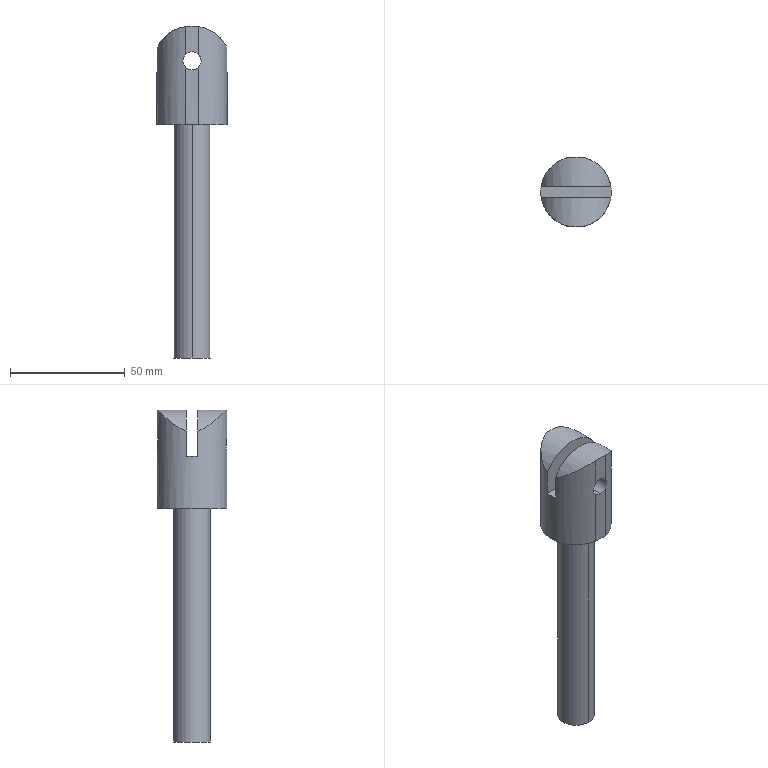Part | NX | features BREP 1 | 1 solid | 20 faces | box 30.734 x 30.163 x 144.78 mm | volume 46621 mm3 | cylinder 11 | plane 9 | commonest cylinder face diameters 7.938 x4 30.734 x3 15.875 x2 34.168 x2
STEP:
#1=CARTESIAN_POINT('',(0.,7.938,-101.6));
#2=VERTEX_POINT('',#1);
#3=CARTESIAN_POINT('',(0.,-7.938,-101.6));
#4=VERTEX_POINT('',#3);
#5=CARTESIAN_POINT('',(0.,0.,-101.6));
#6=DIRECTION('',(0.,0.,-1.));
#7=DIRECTION('',(0.,1.,0.));
#8=AXIS2_PLACEMENT_3D('',#5,#6,#7);
#9=CIRCLE('',#8,7.938);
#10=EDGE_CURVE('',#2,#4,#9,.T.);
#11=ORIENTED_EDGE('',*,*,#10,.T.);
#12=CARTESIAN_POINT('',(0.,0.,-101.6));
#13=DIRECTION('',(0.,0.,-1.));
#14=DIRECTION('',(0.,-1.,0.));
#15=AXIS2_PLACEMENT_3D('',#12,#13,#14);
#16=CIRCLE('',#15,7.938);
#17=EDGE_CURVE('',#4,#2,#16,.T.);
#18=ORIENTED_EDGE('',*,*,#17,.T.);
#19=EDGE_LOOP('',(#11,#18));
#20=FACE_BOUND('',#19,.T.);
#21=CARTESIAN_POINT('',(0.,0.,-101.6));
#22=DIRECTION('',(0.,0.,-1.));
#23=DIRECTION('',(0.,-1.,0.));
#24=AXIS2_PLACEMENT_3D('',#21,#22,#23);
#25=PLANE('',#24);
#26=ADVANCED_FACE('',(#20),#25,.T.);
#27=CARTESIAN_POINT('',(0.,7.938,0.));
#28=VERTEX_POINT('',#27);
#29=CARTESIAN_POINT('',(0.,7.938,0.));
#30=DIRECTION('',(0.,0.,-1.));
#31=VECTOR('',#30,1000.);
#32=LINE('',#29,#31);
#33=EDGE_CURVE('',#2,#28,#32,.F.);
#34=ORIENTED_EDGE('',*,*,#33,.F.);
#35=ORIENTED_EDGE('',*,*,#17,.F.);
#36=CARTESIAN_POINT('',(0.,-7.938,0.));
#37=VERTEX_POINT('',#36);
#38=CARTESIAN_POINT('',(0.,-7.938,0.));
#39=DIRECTION('',(0.,0.,-1.));
#40=VECTOR('',#39,1000.);
#41=LINE('',#38,#40);
#42=EDGE_CURVE('',#4,#37,#41,.F.);
#43=ORIENTED_EDGE('',*,*,#42,.T.);
#44=CARTESIAN_POINT('',(0.,0.,0.));
#45=DIRECTION('',(0.,0.,-1.));
#46=DIRECTION('',(0.,-1.,0.));
#47=AXIS2_PLACEMENT_3D('',#44,#45,#46);
#48=CIRCLE('',#47,7.938);
#49=EDGE_CURVE('',#37,#28,#48,.T.);
#50=ORIENTED_EDGE('',*,*,#49,.T.);
#51=EDGE_LOOP('',(#34,#35,#43,#50));
#52=FACE_BOUND('',#51,.T.);
#53=CARTESIAN_POINT('',(0.,0.,0.));
#54=DIRECTION('',(0.,0.,-1.));
#55=DIRECTION('',(0.,-1.,0.));
#56=AXIS2_PLACEMENT_3D('',#53,#54,#55);
#57=CYLINDRICAL_SURFACE('',#56,7.938);
#58=ADVANCED_FACE('',(#52),#57,.T.);
#59=CARTESIAN_POINT('',(2.95,15.081,0.));
#60=VERTEX_POINT('',#59);
#61=CARTESIAN_POINT('',(-2.95,15.081,0.));
#62=VERTEX_POINT('',#61);
#63=CARTESIAN_POINT('',(2.95,15.081,0.));
#64=DIRECTION('',(-1.,0.,0.));
#65=VECTOR('',#64,1000.);
#66=LINE('',#63,#65);
#67=EDGE_CURVE('',#60,#62,#66,.T.);
#68=ORIENTED_EDGE('',*,*,#67,.F.);
#69=CARTESIAN_POINT('',(15.367,0.,0.));
#70=VERTEX_POINT('',#69);
#71=CARTESIAN_POINT('',(0.,0.,0.));
#72=DIRECTION('',(0.,0.,1.));
#73=DIRECTION('',(0.1919,-0.9814,0.));
#74=AXIS2_PLACEMENT_3D('',#71,#72,#73);
#75=CIRCLE('',#74,15.367);
#76=EDGE_CURVE('',#70,#60,#75,.T.);
#77=ORIENTED_EDGE('',*,*,#76,.F.);
#78=CARTESIAN_POINT('',(2.95,-15.081,0.));
#79=VERTEX_POINT('',#78);
#80=CARTESIAN_POINT('',(0.,0.,0.));
#81=DIRECTION('',(0.,0.,1.));
#82=DIRECTION('',(0.1919,-0.9814,0.));
#83=AXIS2_PLACEMENT_3D('',#80,#81,#82);
#84=CIRCLE('',#83,15.367);
#85=EDGE_CURVE('',#79,#70,#84,.T.);
#86=ORIENTED_EDGE('',*,*,#85,.F.);
#87=CARTESIAN_POINT('',(-2.95,-15.081,0.));
#88=VERTEX_POINT('',#87);
#89=CARTESIAN_POINT('',(-2.95,-15.081,0.));
#90=DIRECTION('',(1.,0.,0.));
#91=VECTOR('',#90,1000.);
#92=LINE('',#89,#91);
#93=EDGE_CURVE('',#88,#79,#92,.T.);
#94=ORIENTED_EDGE('',*,*,#93,.F.);
#95=CARTESIAN_POINT('',(0.,0.,0.));
#96=DIRECTION('',(0.,0.,1.));
#97=DIRECTION('',(-0.1919,0.9814,0.));
#98=AXIS2_PLACEMENT_3D('',#95,#96,#97);
#99=CIRCLE('',#98,15.367);
#100=EDGE_CURVE('',#62,#88,#99,.T.);
#101=ORIENTED_EDGE('',*,*,#100,.F.);
#102=EDGE_LOOP('',(#68,#77,#86,#94,#101));
#103=FACE_BOUND('',#102,.T.);
#104=CARTESIAN_POINT('',(0.,0.,0.));
#105=DIRECTION('',(0.,0.,-1.));
#106=DIRECTION('',(0.,1.,0.));
#107=AXIS2_PLACEMENT_3D('',#104,#105,#106);
#108=CIRCLE('',#107,7.938);
#109=EDGE_CURVE('',#28,#37,#108,.T.);
#110=ORIENTED_EDGE('',*,*,#109,.F.);
#111=ORIENTED_EDGE('',*,*,#49,.F.);
#112=EDGE_LOOP('',(#110,#111));
#113=FACE_BOUND('',#112,.T.);
#114=CARTESIAN_POINT('',(0.,0.,0.));
#115=DIRECTION('',(0.,0.,1.));
#116=DIRECTION('',(1.,0.,0.));
#117=AXIS2_PLACEMENT_3D('',#114,#115,#116);
#118=PLANE('',#117);
#119=ADVANCED_FACE('',(#103,#113),#118,.F.);
#120=CARTESIAN_POINT('',(-2.95,15.081,25.285));
#121=VERTEX_POINT('',#120);
#122=CARTESIAN_POINT('',(-2.95,15.081,0.));
#123=DIRECTION('',(0.,0.,1.));
#124=VECTOR('',#123,1000.);
#125=LINE('',#122,#124);
#126=EDGE_CURVE('',#62,#121,#125,.T.);
#127=ORIENTED_EDGE('',*,*,#126,.F.);
#128=ORIENTED_EDGE('',*,*,#100,.T.);
#129=CARTESIAN_POINT('',(-2.95,-15.081,25.285));
#130=VERTEX_POINT('',#129);
#131=CARTESIAN_POINT('',(-2.95,-15.081,0.));
#132=DIRECTION('',(0.,0.,1.));
#133=VECTOR('',#132,1000.);
#134=LINE('',#131,#133);
#135=EDGE_CURVE('',#88,#130,#134,.T.);
#136=ORIENTED_EDGE('',*,*,#135,.T.);
#137=CARTESIAN_POINT('',(-2.95,-15.081,30.595));
#138=VERTEX_POINT('',#137);
#139=CARTESIAN_POINT('',(-2.95,-15.081,25.285));
#140=CARTESIAN_POINT('',(-3.615,-14.951,26.024));
#141=CARTESIAN_POINT('',(-4.329,-14.739,27.976));
#142=CARTESIAN_POINT('',(-3.601,-14.954,29.872));
#143=CARTESIAN_POINT('',(-2.95,-15.081,30.595));
#144=B_SPLINE_CURVE_WITH_KNOTS('',3,(#139,#140,#141,#142,#143),.UNSPECIFIED.,.F.,.F.,(4,1,4),(0.,0.5,1.),.UNSPECIFIED.);
#145=EDGE_CURVE('',#130,#138,#144,.T.);
#146=ORIENTED_EDGE('',*,*,#145,.T.);
#147=CARTESIAN_POINT('',(-2.95,-15.081,42.923));
#148=VERTEX_POINT('',#147);
#149=CARTESIAN_POINT('',(-2.95,-15.081,30.595));
#150=DIRECTION('',(0.,0.,1.));
#151=VECTOR('',#150,1000.);
#152=LINE('',#149,#151);
#153=EDGE_CURVE('',#138,#148,#152,.T.);
#154=ORIENTED_EDGE('',*,*,#153,.T.);
#155=CARTESIAN_POINT('',(-15.156,-2.54,33.981));
#156=VERTEX_POINT('',#155);
#157=CARTESIAN_POINT('',(-2.95,-15.081,42.923));
#158=CARTESIAN_POINT('',(-3.728,-14.929,42.787));
#159=CARTESIAN_POINT('',(-5.275,-14.509,42.408));
#160=CARTESIAN_POINT('',(-7.248,-13.592,41.602));
#161=CARTESIAN_POINT('',(-8.585,-12.765,40.88));
#162=CARTESIAN_POINT('',(-9.474,-12.114,40.32));
#163=CARTESIAN_POINT('',(-10.176,-11.522,39.82));
#164=CARTESIAN_POINT('',(-10.702,-11.036,39.416));
#165=CARTESIAN_POINT('',(-11.129,-10.603,39.061));
#166=CARTESIAN_POINT('',(-11.433,-10.269,38.791));
#167=CARTESIAN_POINT('',(-11.59,-10.091,38.648));
#168=CARTESIAN_POINT('',(-11.75,-9.904,38.498));
#169=CARTESIAN_POINT('',(-11.744,-9.91,38.503));
#170=CARTESIAN_POINT('',(-11.808,-9.834,38.442));
#171=CARTESIAN_POINT('',(-11.921,-9.699,38.333));
#172=CARTESIAN_POINT('',(-12.171,-9.388,38.085));
#173=CARTESIAN_POINT('',(-12.513,-8.926,37.726));
#174=CARTESIAN_POINT('',(-12.816,-8.484,37.392));
#175=CARTESIAN_POINT('',(-13.102,-8.034,37.059));
#176=CARTESIAN_POINT('',(-13.242,-7.799,36.888));
#177=CARTESIAN_POINT('',(-13.458,-7.424,36.621));
#178=CARTESIAN_POINT('',(-13.68,-7.007,36.332));
#179=CARTESIAN_POINT('',(-13.916,-6.523,36.008));
#180=CARTESIAN_POINT('',(-14.091,-6.138,35.758));
#181=CARTESIAN_POINT('',(-14.311,-5.609,35.431));
#182=CARTESIAN_POINT('',(-14.547,-4.973,35.062));
#183=CARTESIAN_POINT('',(-14.892,-3.882,34.486));
#184=CARTESIAN_POINT('',(-15.07,-3.049,34.145));
#185=CARTESIAN_POINT('',(-15.156,-2.54,33.981));
#186=B_SPLINE_CURVE_WITH_KNOTS('',3,(#157,#158,#159,#160,#161,#162,#163,#164,#165,#166,#167,#168,#169,#170,#171,#172,#173,#174,#175,#176,#177,#178,#179,#180,#181,#182,#183,#184,#185),.UNSPECIFIED.,.F.,.F.,(4,1,1,1,1,1,1,1,1,1,1,1,1,1,1,1,1,1,1,1,1,1,1,1,1,1,4),(0.,0.125,0.25,0.3125,0.375,0.4062,0.4375,0.4688,0.4844,0.4922,0.5,0.5078,0.5156,0.5312,0.5625,0.5938,0.6094,0.625,0.6406,0.6562,0.6875,0.7188,0.75,0.7812,0.8125,0.875,1.),.UNSPECIFIED.);
#187=EDGE_CURVE('',#156,#148,#186,.F.);
#188=ORIENTED_EDGE('',*,*,#187,.F.);
#189=CARTESIAN_POINT('',(-15.156,-2.54,22.965));
#190=VERTEX_POINT('',#189);
#191=CARTESIAN_POINT('',(-15.156,-2.54,22.965));
#192=DIRECTION('',(0.,0.,1.));
#193=VECTOR('',#192,1000.);
#194=LINE('',#191,#193);
#195=EDGE_CURVE('',#190,#156,#194,.T.);
#196=ORIENTED_EDGE('',*,*,#195,.F.);
#197=CARTESIAN_POINT('',(-15.156,2.54,22.965));
#198=VERTEX_POINT('',#197);
#199=CARTESIAN_POINT('',(0.,0.,22.965));
#200=DIRECTION('',(0.,0.,1.));
#201=DIRECTION('',(-0.9862,0.1653,0.));
#202=AXIS2_PLACEMENT_3D('',#199,#200,#201);
#203=CIRCLE('',#202,15.367);
#204=EDGE_CURVE('',#198,#190,#203,.T.);
#205=ORIENTED_EDGE('',*,*,#204,.F.);
#206=CARTESIAN_POINT('',(-15.156,2.54,33.981));
#207=VERTEX_POINT('',#206);
#208=CARTESIAN_POINT('',(-15.156,2.54,22.965));
#209=DIRECTION('',(0.,0.,1.));
#210=VECTOR('',#209,1000.);
#211=LINE('',#208,#210);
#212=EDGE_CURVE('',#198,#207,#211,.T.);
#213=ORIENTED_EDGE('',*,*,#212,.T.);
#214=CARTESIAN_POINT('',(-2.95,15.081,42.923));
#215=VERTEX_POINT('',#214);
#216=CARTESIAN_POINT('',(-15.156,2.54,33.981));
#217=CARTESIAN_POINT('',(-15.07,3.049,34.145));
#218=CARTESIAN_POINT('',(-14.886,3.896,34.495));
#219=CARTESIAN_POINT('',(-14.508,5.105,35.129));
#220=CARTESIAN_POINT('',(-14.158,5.99,35.662));
#221=CARTESIAN_POINT('',(-13.916,6.525,36.009));
#222=CARTESIAN_POINT('',(-13.68,7.007,36.331));
#223=CARTESIAN_POINT('',(-13.458,7.424,36.621));
#224=CARTESIAN_POINT('',(-13.242,7.799,36.889));
#225=CARTESIAN_POINT('',(-13.105,8.03,37.056));
#226=CARTESIAN_POINT('',(-12.81,8.493,37.399));
#227=CARTESIAN_POINT('',(-12.503,8.94,37.737));
#228=CARTESIAN_POINT('',(-12.157,9.406,38.098));
#229=CARTESIAN_POINT('',(-11.911,9.71,38.342));
#230=CARTESIAN_POINT('',(-11.806,9.837,38.444));
#231=CARTESIAN_POINT('',(-11.747,9.907,38.501));
#232=CARTESIAN_POINT('',(-11.759,9.894,38.49));
#233=CARTESIAN_POINT('',(-11.597,10.084,38.642));
#234=CARTESIAN_POINT('',(-11.44,10.261,38.785));
#235=CARTESIAN_POINT('',(-11.134,10.597,39.057));
#236=CARTESIAN_POINT('',(-10.706,11.032,39.413));
#237=CARTESIAN_POINT('',(-10.178,11.521,39.82));
#238=CARTESIAN_POINT('',(-9.471,12.117,40.322));
#239=CARTESIAN_POINT('',(-8.576,12.771,40.885));
#240=CARTESIAN_POINT('',(-7.219,13.608,41.616));
#241=CARTESIAN_POINT('',(-5.268,14.509,42.409));
#242=CARTESIAN_POINT('',(-3.725,14.93,42.787));
#243=CARTESIAN_POINT('',(-2.95,15.081,42.923));
#244=B_SPLINE_CURVE_WITH_KNOTS('',3,(#216,#217,#218,#219,#220,#221,#222,#223,#224,#225,#226,#227,#228,#229,#230,#231,#232,#233,#234,#235,#236,#237,#238,#239,#240,#241,#242,#243),.UNSPECIFIED.,.F.,.F.,(4,1,1,1,1,1,1,1,1,1,1,1,1,1,1,1,1,1,1,1,1,1,1,1,1,4),(0.,0.125,0.1875,0.25,0.2812,0.3125,0.3438,0.3594,0.375,0.3906,0.4062,0.4375,0.4688,0.4844,0.4922,0.5,0.5078,0.5156,0.5312,0.5625,0.5938,0.625,0.6875,0.75,0.875,1.),.UNSPECIFIED.);
#245=EDGE_CURVE('',#215,#207,#244,.F.);
#246=ORIENTED_EDGE('',*,*,#245,.F.);
#247=CARTESIAN_POINT('',(-2.95,15.081,30.595));
#248=VERTEX_POINT('',#247);
#249=CARTESIAN_POINT('',(-2.95,15.081,30.595));
#250=DIRECTION('',(0.,0.,1.));
#251=VECTOR('',#250,1000.);
#252=LINE('',#249,#251);
#253=EDGE_CURVE('',#248,#215,#252,.T.);
#254=ORIENTED_EDGE('',*,*,#253,.F.);
#255=CARTESIAN_POINT('',(-2.95,15.081,30.595));
#256=CARTESIAN_POINT('',(-3.602,14.954,29.87));
#257=CARTESIAN_POINT('',(-4.33,14.739,27.965));
#258=CARTESIAN_POINT('',(-3.612,14.952,26.021));
#259=CARTESIAN_POINT('',(-2.95,15.081,25.285));
#260=B_SPLINE_CURVE_WITH_KNOTS('',3,(#255,#256,#257,#258,#259),.UNSPECIFIED.,.F.,.F.,(4,1,4),(0.,0.5,1.),.UNSPECIFIED.);
#261=EDGE_CURVE('',#248,#121,#260,.T.);
#262=ORIENTED_EDGE('',*,*,#261,.T.);
#263=EDGE_LOOP('',(#127,#128,#136,#146,#154,#188,#196,#205,#213,#246,#254,#262));
#264=FACE_BOUND('',#263,.T.);
#265=CARTESIAN_POINT('',(0.,0.,0.));
#266=DIRECTION('',(0.,0.,1.));
#267=DIRECTION('',(1.,0.,0.));
#268=AXIS2_PLACEMENT_3D('',#265,#266,#267);
#269=CYLINDRICAL_SURFACE('',#268,15.367);
#270=ADVANCED_FACE('',(#264),#269,.T.);
#271=CARTESIAN_POINT('',(0.,-15.081,31.909));
#272=VERTEX_POINT('',#271);
#273=CARTESIAN_POINT('',(0.,-2.54,31.909));
#274=VERTEX_POINT('',#273);
#275=CARTESIAN_POINT('',(0.,-2.54,31.909));
#276=DIRECTION('',(0.,-1.,0.));
#277=VECTOR('',#276,1000.);
#278=LINE('',#275,#277);
#279=EDGE_CURVE('',#272,#274,#278,.F.);
#280=ORIENTED_EDGE('',*,*,#279,.F.);
#281=CARTESIAN_POINT('',(0.,-15.081,27.94));
#282=DIRECTION('',(0.,1.,0.));
#283=DIRECTION('',(-0.7432,0.,0.669));
#284=AXIS2_PLACEMENT_3D('',#281,#282,#283);
#285=CIRCLE('',#284,3.969);
#286=EDGE_CURVE('',#138,#272,#285,.T.);
#287=ORIENTED_EDGE('',*,*,#286,.F.);
#288=ORIENTED_EDGE('',*,*,#145,.F.);
#289=CARTESIAN_POINT('',(0.,-15.081,23.971));
#290=VERTEX_POINT('',#289);
#291=CARTESIAN_POINT('',(0.,-15.081,27.94));
#292=DIRECTION('',(0.,1.,0.));
#293=DIRECTION('',(0.,0.,-1.));
#294=AXIS2_PLACEMENT_3D('',#291,#292,#293);
#295=CIRCLE('',#294,3.969);
#296=EDGE_CURVE('',#290,#130,#295,.T.);
#297=ORIENTED_EDGE('',*,*,#296,.F.);
#298=CARTESIAN_POINT('',(0.,-2.54,23.971));
#299=VERTEX_POINT('',#298);
#300=CARTESIAN_POINT('',(0.,-2.54,23.971));
#301=DIRECTION('',(0.,-1.,0.));
#302=VECTOR('',#301,1000.);
#303=LINE('',#300,#302);
#304=EDGE_CURVE('',#290,#299,#303,.F.);
#305=ORIENTED_EDGE('',*,*,#304,.T.);
#306=CARTESIAN_POINT('',(0.,-2.54,27.94));
#307=DIRECTION('',(0.,1.,0.));
#308=DIRECTION('',(0.,0.,-1.));
#309=AXIS2_PLACEMENT_3D('',#306,#307,#308);
#310=CIRCLE('',#309,3.969);
#311=EDGE_CURVE('',#299,#274,#310,.T.);
#312=ORIENTED_EDGE('',*,*,#311,.T.);
#313=EDGE_LOOP('',(#280,#287,#288,#297,#305,#312));
#314=FACE_BOUND('',#313,.T.);
#315=CARTESIAN_POINT('',(0.,18.098,27.94));
#316=DIRECTION('',(0.,1.,0.));
#317=DIRECTION('',(0.,0.,-1.));
#318=AXIS2_PLACEMENT_3D('',#315,#316,#317);
#319=CYLINDRICAL_SURFACE('',#318,3.969);
#320=ADVANCED_FACE('',(#314),#319,.F.);
#321=CARTESIAN_POINT('',(0.,15.081,23.971));
#322=VERTEX_POINT('',#321);
#323=CARTESIAN_POINT('',(0.,2.54,23.971));
#324=VERTEX_POINT('',#323);
#325=CARTESIAN_POINT('',(0.,15.081,23.971));
#326=DIRECTION('',(0.,-1.,0.));
#327=VECTOR('',#326,1000.);
#328=LINE('',#325,#327);
#329=EDGE_CURVE('',#322,#324,#328,.T.);
#330=ORIENTED_EDGE('',*,*,#329,.F.);
#331=CARTESIAN_POINT('',(0.,15.081,27.94));
#332=DIRECTION('',(0.,1.,0.));
#333=DIRECTION('',(0.,0.,-1.));
#334=AXIS2_PLACEMENT_3D('',#331,#332,#333);
#335=CIRCLE('',#334,3.969);
#336=EDGE_CURVE('',#322,#121,#335,.T.);
#337=ORIENTED_EDGE('',*,*,#336,.T.);
#338=ORIENTED_EDGE('',*,*,#261,.F.);
#339=CARTESIAN_POINT('',(0.,15.081,31.909));
#340=VERTEX_POINT('',#339);
#341=CARTESIAN_POINT('',(0.,15.081,27.94));
#342=DIRECTION('',(0.,1.,0.));
#343=DIRECTION('',(-0.7432,0.,0.669));
#344=AXIS2_PLACEMENT_3D('',#341,#342,#343);
#345=CIRCLE('',#344,3.969);
#346=EDGE_CURVE('',#248,#340,#345,.T.);
#347=ORIENTED_EDGE('',*,*,#346,.T.);
#348=CARTESIAN_POINT('',(0.,2.54,31.909));
#349=VERTEX_POINT('',#348);
#350=CARTESIAN_POINT('',(0.,15.081,31.909));
#351=DIRECTION('',(0.,-1.,0.));
#352=VECTOR('',#351,1000.);
#353=LINE('',#350,#352);
#354=EDGE_CURVE('',#340,#349,#353,.T.);
#355=ORIENTED_EDGE('',*,*,#354,.T.);
#356=CARTESIAN_POINT('',(0.,2.54,27.94));
#357=DIRECTION('',(0.,1.,0.));
#358=DIRECTION('',(0.,0.,-1.));
#359=AXIS2_PLACEMENT_3D('',#356,#357,#358);
#360=CIRCLE('',#359,3.969);
#361=EDGE_CURVE('',#324,#349,#360,.T.);
#362=ORIENTED_EDGE('',*,*,#361,.F.);
#363=EDGE_LOOP('',(#330,#337,#338,#347,#355,#362));
#364=FACE_BOUND('',#363,.T.);
#365=CARTESIAN_POINT('',(0.,18.098,27.94));
#366=DIRECTION('',(0.,1.,0.));
#367=DIRECTION('',(0.,0.,-1.));
#368=AXIS2_PLACEMENT_3D('',#365,#366,#367);
#369=CYLINDRICAL_SURFACE('',#368,3.969);
#370=ADVANCED_FACE('',(#364),#369,.F.);
#371=CARTESIAN_POINT('',(15.156,-2.54,22.965));
#372=VERTEX_POINT('',#371);
#373=CARTESIAN_POINT('',(15.156,-2.54,33.981));
#374=VERTEX_POINT('',#373);
#375=CARTESIAN_POINT('',(15.156,-2.54,22.965));
#376=DIRECTION('',(0.,0.,1.));
#377=VECTOR('',#376,1000.);
#378=LINE('',#375,#377);
#379=EDGE_CURVE('',#372,#374,#378,.T.);
#380=ORIENTED_EDGE('',*,*,#379,.F.);
#381=CARTESIAN_POINT('',(15.156,-2.54,22.965));
#382=DIRECTION('',(-1.,0.,0.));
#383=VECTOR('',#382,1000.);
#384=LINE('',#381,#383);
#385=EDGE_CURVE('',#372,#190,#384,.T.);
#386=ORIENTED_EDGE('',*,*,#385,.T.);
#387=ORIENTED_EDGE('',*,*,#195,.T.);
#388=CARTESIAN_POINT('',(0.,-2.54,26.096));
#389=DIRECTION('',(0.,1.,0.));
#390=DIRECTION('',(-0.8871,0.,0.4616));
#391=AXIS2_PLACEMENT_3D('',#388,#389,#390);
#392=CIRCLE('',#391,17.084);
#393=EDGE_CURVE('',#156,#374,#392,.T.);
#394=ORIENTED_EDGE('',*,*,#393,.T.);
#395=EDGE_LOOP('',(#380,#386,#387,#394));
#396=FACE_BOUND('',#395,.T.);
#397=CARTESIAN_POINT('',(0.,-2.54,27.94));
#398=DIRECTION('',(0.,1.,0.));
#399=DIRECTION('',(0.,0.,1.));
#400=AXIS2_PLACEMENT_3D('',#397,#398,#399);
#401=CIRCLE('',#400,3.969);
#402=EDGE_CURVE('',#274,#299,#401,.T.);
#403=ORIENTED_EDGE('',*,*,#402,.F.);
#404=ORIENTED_EDGE('',*,*,#311,.F.);
#405=EDGE_LOOP('',(#403,#404));
#406=FACE_BOUND('',#405,.T.);
#407=CARTESIAN_POINT('',(18.44,-2.54,43.18));
#408=DIRECTION('',(0.,-1.,0.));
#409=DIRECTION('',(0.,0.,-1.));
#410=AXIS2_PLACEMENT_3D('',#407,#408,#409);
#411=PLANE('',#410);
#412=ADVANCED_FACE('',(#396,#406),#411,.F.);
#413=ORIENTED_EDGE('',*,*,#187,.T.);
#414=CARTESIAN_POINT('',(2.95,-15.081,42.923));
#415=VERTEX_POINT('',#414);
#416=CARTESIAN_POINT('',(0.,-15.081,26.096));
#417=DIRECTION('',(0.,1.,0.));
#418=DIRECTION('',(-0.1727,0.,0.985));
#419=AXIS2_PLACEMENT_3D('',#416,#417,#418);
#420=CIRCLE('',#419,17.084);
#421=EDGE_CURVE('',#148,#415,#420,.T.);
#422=ORIENTED_EDGE('',*,*,#421,.T.);
#423=CARTESIAN_POINT('',(2.95,-15.081,42.923));
#424=CARTESIAN_POINT('',(3.745,-14.926,42.784));
#425=CARTESIAN_POINT('',(5.335,-14.477,42.382));
#426=CARTESIAN_POINT('',(7.142,-13.656,41.656));
#427=CARTESIAN_POINT('',(8.702,-12.691,40.818));
#428=CARTESIAN_POINT('',(9.783,-11.875,40.12));
#429=CARTESIAN_POINT('',(10.786,-10.977,39.367));
#430=CARTESIAN_POINT('',(11.783,-9.892,38.484));
#431=CARTESIAN_POINT('',(12.455,-9.026,37.801));
#432=CARTESIAN_POINT('',(13.307,-7.762,36.844));
#433=CARTESIAN_POINT('',(14.167,-6.071,35.681));
#434=CARTESIAN_POINT('',(14.799,-4.273,34.651));
#435=CARTESIAN_POINT('',(15.061,-3.106,34.163));
#436=CARTESIAN_POINT('',(15.156,-2.54,33.981));
#437=B_SPLINE_CURVE_WITH_KNOTS('',3,(#423,#424,#425,#426,#427,#428,#429,#430,#431,#432,#433,#434,#435,#436),.UNSPECIFIED.,.F.,.F.,(4,1,1,1,1,1,1,1,1,1,1,4),(0.,0.125,0.25,0.3125,0.375,0.4375,0.5,0.5625,0.625,0.75,0.875,1.),.UNSPECIFIED.);
#438=EDGE_CURVE('',#415,#374,#437,.T.);
#439=ORIENTED_EDGE('',*,*,#438,.T.);
#440=ORIENTED_EDGE('',*,*,#393,.F.);
#441=EDGE_LOOP('',(#413,#422,#439,#440));
#442=FACE_BOUND('',#441,.T.);
#443=CARTESIAN_POINT('',(0.,18.098,26.096));
#444=DIRECTION('',(0.,1.,0.));
#445=DIRECTION('',(1.,0.,0.));
#446=AXIS2_PLACEMENT_3D('',#443,#444,#445);
#447=CYLINDRICAL_SURFACE('',#446,17.084);
#448=ADVANCED_FACE('',(#442),#447,.T.);
#449=CARTESIAN_POINT('',(15.156,2.54,33.981));
#450=VERTEX_POINT('',#449);
#451=CARTESIAN_POINT('',(2.95,15.081,42.923));
#452=VERTEX_POINT('',#451);
#453=CARTESIAN_POINT('',(15.156,2.54,33.981));
#454=CARTESIAN_POINT('',(14.966,3.672,34.346));
#455=CARTESIAN_POINT('',(14.499,5.42,35.232));
#456=CARTESIAN_POINT('',(13.306,7.763,36.846));
#457=CARTESIAN_POINT('',(12.453,9.029,37.804));
#458=CARTESIAN_POINT('',(11.771,9.907,38.496));
#459=CARTESIAN_POINT('',(10.791,10.972,39.363));
#460=CARTESIAN_POINT('',(9.795,11.865,40.111));
#461=CARTESIAN_POINT('',(8.722,12.677,40.806));
#462=CARTESIAN_POINT('',(7.166,13.644,41.646));
#463=CARTESIAN_POINT('',(5.35,14.473,42.378));
#464=CARTESIAN_POINT('',(3.752,14.924,42.783));
#465=CARTESIAN_POINT('',(2.95,15.081,42.923));
#466=B_SPLINE_CURVE_WITH_KNOTS('',3,(#453,#454,#455,#456,#457,#458,#459,#460,#461,#462,#463,#464,#465),.UNSPECIFIED.,.F.,.F.,(4,1,1,1,1,1,1,1,1,1,4),(0.,0.25,0.375,0.4375,0.5,0.5625,0.625,0.6875,0.75,0.875,1.),.UNSPECIFIED.);
#467=EDGE_CURVE('',#450,#452,#466,.T.);
#468=ORIENTED_EDGE('',*,*,#467,.T.);
#469=CARTESIAN_POINT('',(0.,15.081,26.096));
#470=DIRECTION('',(0.,-1.,0.));
#471=DIRECTION('',(0.1727,0.,0.985));
#472=AXIS2_PLACEMENT_3D('',#469,#470,#471);
#473=CIRCLE('',#472,17.084);
#474=EDGE_CURVE('',#452,#215,#473,.T.);
#475=ORIENTED_EDGE('',*,*,#474,.T.);
#476=ORIENTED_EDGE('',*,*,#245,.T.);
#477=CARTESIAN_POINT('',(0.,2.54,26.096));
#478=DIRECTION('',(0.,1.,0.));
#479=DIRECTION('',(-0.8871,0.,0.4616));
#480=AXIS2_PLACEMENT_3D('',#477,#478,#479);
#481=CIRCLE('',#480,17.084);
#482=EDGE_CURVE('',#207,#450,#481,.T.);
#483=ORIENTED_EDGE('',*,*,#482,.T.);
#484=EDGE_LOOP('',(#468,#475,#476,#483));
#485=FACE_BOUND('',#484,.T.);
#486=CARTESIAN_POINT('',(0.,18.098,26.096));
#487=DIRECTION('',(0.,1.,0.));
#488=DIRECTION('',(1.,0.,0.));
#489=AXIS2_PLACEMENT_3D('',#486,#487,#488);
#490=CYLINDRICAL_SURFACE('',#489,17.084);
#491=ADVANCED_FACE('',(#485),#490,.T.);
#492=CARTESIAN_POINT('',(15.367,0.,22.965));
#493=VERTEX_POINT('',#492);
#494=CARTESIAN_POINT('',(15.367,0.,0.));
#495=DIRECTION('',(0.,0.,1.));
#496=VECTOR('',#495,1000.);
#497=LINE('',#494,#496);
#498=EDGE_CURVE('',#70,#493,#497,.T.);
#499=ORIENTED_EDGE('',*,*,#498,.F.);
#500=ORIENTED_EDGE('',*,*,#76,.T.);
#501=CARTESIAN_POINT('',(2.95,15.081,25.285));
#502=VERTEX_POINT('',#501);
#503=CARTESIAN_POINT('',(2.95,15.081,0.));
#504=DIRECTION('',(0.,0.,1.));
#505=VECTOR('',#504,1000.);
#506=LINE('',#503,#505);
#507=EDGE_CURVE('',#60,#502,#506,.T.);
#508=ORIENTED_EDGE('',*,*,#507,.T.);
#509=CARTESIAN_POINT('',(2.95,15.081,30.595));
#510=VERTEX_POINT('',#509);
#511=CARTESIAN_POINT('',(2.95,15.081,25.285));
#512=CARTESIAN_POINT('',(3.601,14.954,26.008));
#513=CARTESIAN_POINT('',(4.329,14.739,27.908));
#514=CARTESIAN_POINT('',(3.615,14.951,29.856));
#515=CARTESIAN_POINT('',(2.95,15.081,30.595));
#516=B_SPLINE_CURVE_WITH_KNOTS('',3,(#511,#512,#513,#514,#515),.UNSPECIFIED.,.F.,.F.,(4,1,4),(0.,0.5,1.),.UNSPECIFIED.);
#517=EDGE_CURVE('',#502,#510,#516,.T.);
#518=ORIENTED_EDGE('',*,*,#517,.T.);
#519=CARTESIAN_POINT('',(2.95,15.081,30.595));
#520=DIRECTION('',(0.,0.,1.));
#521=VECTOR('',#520,1000.);
#522=LINE('',#519,#521);
#523=EDGE_CURVE('',#510,#452,#522,.T.);
#524=ORIENTED_EDGE('',*,*,#523,.T.);
#525=ORIENTED_EDGE('',*,*,#467,.F.);
#526=CARTESIAN_POINT('',(15.156,2.54,22.965));
#527=VERTEX_POINT('',#526);
#528=CARTESIAN_POINT('',(15.156,2.54,22.965));
#529=DIRECTION('',(0.,0.,1.));
#530=VECTOR('',#529,1000.);
#531=LINE('',#528,#530);
#532=EDGE_CURVE('',#527,#450,#531,.T.);
#533=ORIENTED_EDGE('',*,*,#532,.F.);
#534=CARTESIAN_POINT('',(0.,0.,22.965));
#535=DIRECTION('',(0.,0.,1.));
#536=DIRECTION('',(0.9862,-0.1653,0.));
#537=AXIS2_PLACEMENT_3D('',#534,#535,#536);
#538=CIRCLE('',#537,15.367);
#539=EDGE_CURVE('',#493,#527,#538,.T.);
#540=ORIENTED_EDGE('',*,*,#539,.F.);
#541=EDGE_LOOP('',(#499,#500,#508,#518,#524,#525,#533,#540));
#542=FACE_BOUND('',#541,.T.);
#543=CARTESIAN_POINT('',(0.,0.,0.));
#544=DIRECTION('',(0.,0.,1.));
#545=DIRECTION('',(1.,0.,0.));
#546=AXIS2_PLACEMENT_3D('',#543,#544,#545);
#547=CYLINDRICAL_SURFACE('',#546,15.367);
#548=ADVANCED_FACE('',(#542),#547,.T.);
#549=ORIENTED_EDGE('',*,*,#304,.F.);
#550=CARTESIAN_POINT('',(2.95,-15.081,25.285));
#551=VERTEX_POINT('',#550);
#552=CARTESIAN_POINT('',(0.,-15.081,27.94));
#553=DIRECTION('',(0.,1.,0.));
#554=DIRECTION('',(0.7432,0.,-0.669));
#555=AXIS2_PLACEMENT_3D('',#552,#553,#554);
#556=CIRCLE('',#555,3.969);
#557=EDGE_CURVE('',#551,#290,#556,.T.);
#558=ORIENTED_EDGE('',*,*,#557,.F.);
#559=CARTESIAN_POINT('',(2.95,-15.081,30.595));
#560=VERTEX_POINT('',#559);
#561=CARTESIAN_POINT('',(2.95,-15.081,25.285));
#562=CARTESIAN_POINT('',(3.151,-15.042,25.508));
#563=CARTESIAN_POINT('',(3.468,-14.973,25.976));
#564=CARTESIAN_POINT('',(3.701,-14.915,26.455));
#565=CARTESIAN_POINT('',(3.933,-14.856,27.235));
#566=CARTESIAN_POINT('',(3.986,-14.841,27.92));
#567=CARTESIAN_POINT('',(3.937,-14.855,28.618));
#568=CARTESIAN_POINT('',(3.715,-14.911,29.389));
#569=CARTESIAN_POINT('',(3.476,-14.971,29.893));
#570=CARTESIAN_POINT('',(3.154,-15.041,30.368));
#571=CARTESIAN_POINT('',(2.95,-15.081,30.595));
#572=B_SPLINE_CURVE_WITH_KNOTS('',3,(#561,#562,#563,#564,#565,#566,#567,#568,#569,#570,#571),.UNSPECIFIED.,.F.,.F.,(4,1,1,1,1,1,1,1,4),(0.,0.125,0.25,0.375,0.5,0.625,0.75,0.875,1.),.UNSPECIFIED.);
#573=EDGE_CURVE('',#560,#551,#572,.F.);
#574=ORIENTED_EDGE('',*,*,#573,.F.);
#575=CARTESIAN_POINT('',(0.,-15.081,27.94));
#576=DIRECTION('',(0.,1.,0.));
#577=DIRECTION('',(0.,0.,1.));
#578=AXIS2_PLACEMENT_3D('',#575,#576,#577);
#579=CIRCLE('',#578,3.969);
#580=EDGE_CURVE('',#272,#560,#579,.T.);
#581=ORIENTED_EDGE('',*,*,#580,.F.);
#582=ORIENTED_EDGE('',*,*,#279,.T.);
#583=ORIENTED_EDGE('',*,*,#402,.T.);
#584=EDGE_LOOP('',(#549,#558,#574,#581,#582,#583));
#585=FACE_BOUND('',#584,.T.);
#586=CARTESIAN_POINT('',(0.,18.098,27.94));
#587=DIRECTION('',(0.,1.,0.));
#588=DIRECTION('',(0.,0.,-1.));
#589=AXIS2_PLACEMENT_3D('',#586,#587,#588);
#590=CYLINDRICAL_SURFACE('',#589,3.969);
#591=ADVANCED_FACE('',(#585),#590,.F.);
#592=ORIENTED_EDGE('',*,*,#354,.F.);
#593=CARTESIAN_POINT('',(0.,15.081,27.94));
#594=DIRECTION('',(0.,1.,0.));
#595=DIRECTION('',(0.,0.,1.));
#596=AXIS2_PLACEMENT_3D('',#593,#594,#595);
#597=CIRCLE('',#596,3.969);
#598=EDGE_CURVE('',#340,#510,#597,.T.);
#599=ORIENTED_EDGE('',*,*,#598,.T.);
#600=ORIENTED_EDGE('',*,*,#517,.F.);
#601=CARTESIAN_POINT('',(0.,15.081,27.94));
#602=DIRECTION('',(0.,1.,0.));
#603=DIRECTION('',(0.7432,0.,-0.669));
#604=AXIS2_PLACEMENT_3D('',#601,#602,#603);
#605=CIRCLE('',#604,3.969);
#606=EDGE_CURVE('',#502,#322,#605,.T.);
#607=ORIENTED_EDGE('',*,*,#606,.T.);
#608=ORIENTED_EDGE('',*,*,#329,.T.);
#609=CARTESIAN_POINT('',(0.,2.54,27.94));
#610=DIRECTION('',(0.,1.,0.));
#611=DIRECTION('',(0.,0.,1.));
#612=AXIS2_PLACEMENT_3D('',#609,#610,#611);
#613=CIRCLE('',#612,3.969);
#614=EDGE_CURVE('',#349,#324,#613,.T.);
#615=ORIENTED_EDGE('',*,*,#614,.F.);
#616=EDGE_LOOP('',(#592,#599,#600,#607,#608,#615));
#617=FACE_BOUND('',#616,.T.);
#618=CARTESIAN_POINT('',(0.,18.098,27.94));
#619=DIRECTION('',(0.,1.,0.));
#620=DIRECTION('',(0.,0.,-1.));
#621=AXIS2_PLACEMENT_3D('',#618,#619,#620);
#622=CYLINDRICAL_SURFACE('',#621,3.969);
#623=ADVANCED_FACE('',(#617),#622,.F.);
#624=ORIENTED_EDGE('',*,*,#135,.F.);
#625=ORIENTED_EDGE('',*,*,#93,.T.);
#626=CARTESIAN_POINT('',(2.95,-15.081,0.));
#627=DIRECTION('',(0.,0.,1.));
#628=VECTOR('',#627,1000.);
#629=LINE('',#626,#628);
#630=EDGE_CURVE('',#79,#551,#629,.T.);
#631=ORIENTED_EDGE('',*,*,#630,.T.);
#632=ORIENTED_EDGE('',*,*,#557,.T.);
#633=ORIENTED_EDGE('',*,*,#296,.T.);
#634=EDGE_LOOP('',(#624,#625,#631,#632,#633));
#635=FACE_BOUND('',#634,.T.);
#636=CARTESIAN_POINT('',(-2.95,-15.081,0.));
#637=DIRECTION('',(0.,-1.,0.));
#638=DIRECTION('',(0.,0.,-1.));
#639=AXIS2_PLACEMENT_3D('',#636,#637,#638);
#640=PLANE('',#639);
#641=ADVANCED_FACE('',(#635),#640,.T.);
#642=ORIENTED_EDGE('',*,*,#580,.T.);
#643=CARTESIAN_POINT('',(2.95,-15.081,30.595));
#644=DIRECTION('',(0.,0.,1.));
#645=VECTOR('',#644,1000.);
#646=LINE('',#643,#645);
#647=EDGE_CURVE('',#560,#415,#646,.T.);
#648=ORIENTED_EDGE('',*,*,#647,.T.);
#649=ORIENTED_EDGE('',*,*,#421,.F.);
#650=ORIENTED_EDGE('',*,*,#153,.F.);
#651=ORIENTED_EDGE('',*,*,#286,.T.);
#652=EDGE_LOOP('',(#642,#648,#649,#650,#651));
#653=FACE_BOUND('',#652,.T.);
#654=CARTESIAN_POINT('',(-2.95,-15.081,0.));
#655=DIRECTION('',(0.,-1.,0.));
#656=DIRECTION('',(0.,0.,-1.));
#657=AXIS2_PLACEMENT_3D('',#654,#655,#656);
#658=PLANE('',#657);
#659=ADVANCED_FACE('',(#653),#658,.T.);
#660=ORIENTED_EDGE('',*,*,#212,.F.);
#661=CARTESIAN_POINT('',(15.156,2.54,22.965));
#662=DIRECTION('',(-1.,0.,0.));
#663=VECTOR('',#662,1000.);
#664=LINE('',#661,#663);
#665=EDGE_CURVE('',#527,#198,#664,.T.);
#666=ORIENTED_EDGE('',*,*,#665,.F.);
#667=ORIENTED_EDGE('',*,*,#532,.T.);
#668=ORIENTED_EDGE('',*,*,#482,.F.);
#669=EDGE_LOOP('',(#660,#666,#667,#668));
#670=FACE_BOUND('',#669,.T.);
#671=ORIENTED_EDGE('',*,*,#614,.T.);
#672=ORIENTED_EDGE('',*,*,#361,.T.);
#673=EDGE_LOOP('',(#671,#672));
#674=FACE_BOUND('',#673,.T.);
#675=CARTESIAN_POINT('',(18.44,2.54,22.965));
#676=DIRECTION('',(0.,1.,0.));
#677=DIRECTION('',(1.,0.,0.));
#678=AXIS2_PLACEMENT_3D('',#675,#676,#677);
#679=PLANE('',#678);
#680=ADVANCED_FACE('',(#670,#674),#679,.F.);
#681=CARTESIAN_POINT('',(0.,0.,22.965));
#682=DIRECTION('',(0.,0.,1.));
#683=DIRECTION('',(0.9862,-0.1653,0.));
#684=AXIS2_PLACEMENT_3D('',#681,#682,#683);
#685=CIRCLE('',#684,15.367);
#686=EDGE_CURVE('',#372,#493,#685,.T.);
#687=ORIENTED_EDGE('',*,*,#686,.T.);
#688=ORIENTED_EDGE('',*,*,#539,.T.);
#689=ORIENTED_EDGE('',*,*,#665,.T.);
#690=ORIENTED_EDGE('',*,*,#204,.T.);
#691=ORIENTED_EDGE('',*,*,#385,.F.);
#692=EDGE_LOOP('',(#687,#688,#689,#690,#691));
#693=FACE_BOUND('',#692,.T.);
#694=CARTESIAN_POINT('',(18.44,-2.54,22.965));
#695=DIRECTION('',(0.,0.,-1.));
#696=DIRECTION('',(0.,-1.,0.));
#697=AXIS2_PLACEMENT_3D('',#694,#695,#696);
#698=PLANE('',#697);
#699=ADVANCED_FACE('',(#693),#698,.F.);
#700=ORIENTED_EDGE('',*,*,#606,.F.);
#701=ORIENTED_EDGE('',*,*,#507,.F.);
#702=ORIENTED_EDGE('',*,*,#67,.T.);
#703=ORIENTED_EDGE('',*,*,#126,.T.);
#704=ORIENTED_EDGE('',*,*,#336,.F.);
#705=EDGE_LOOP('',(#700,#701,#702,#703,#704));
#706=FACE_BOUND('',#705,.T.);
#707=CARTESIAN_POINT('',(2.95,15.081,0.));
#708=DIRECTION('',(0.,1.,0.));
#709=DIRECTION('',(1.,0.,0.));
#710=AXIS2_PLACEMENT_3D('',#707,#708,#709);
#711=PLANE('',#710);
#712=ADVANCED_FACE('',(#706),#711,.T.);
#713=ORIENTED_EDGE('',*,*,#253,.T.);
#714=ORIENTED_EDGE('',*,*,#474,.F.);
#715=ORIENTED_EDGE('',*,*,#523,.F.);
#716=ORIENTED_EDGE('',*,*,#598,.F.);
#717=ORIENTED_EDGE('',*,*,#346,.F.);
#718=EDGE_LOOP('',(#713,#714,#715,#716,#717));
#719=FACE_BOUND('',#718,.T.);
#720=CARTESIAN_POINT('',(2.95,15.081,0.));
#721=DIRECTION('',(0.,1.,0.));
#722=DIRECTION('',(1.,0.,0.));
#723=AXIS2_PLACEMENT_3D('',#720,#721,#722);
#724=PLANE('',#723);
#725=ADVANCED_FACE('',(#719),#724,.T.);
#726=ORIENTED_EDGE('',*,*,#42,.F.);
#727=ORIENTED_EDGE('',*,*,#10,.F.);
#728=ORIENTED_EDGE('',*,*,#33,.T.);
#729=ORIENTED_EDGE('',*,*,#109,.T.);
#730=EDGE_LOOP('',(#726,#727,#728,#729));
#731=FACE_BOUND('',#730,.T.);
#732=CARTESIAN_POINT('',(0.,0.,0.));
#733=DIRECTION('',(0.,0.,-1.));
#734=DIRECTION('',(0.,-1.,0.));
#735=AXIS2_PLACEMENT_3D('',#732,#733,#734);
#736=CYLINDRICAL_SURFACE('',#735,7.938);
#737=ADVANCED_FACE('',(#731),#736,.T.);
#738=ORIENTED_EDGE('',*,*,#85,.T.);
#739=ORIENTED_EDGE('',*,*,#498,.T.);
#740=ORIENTED_EDGE('',*,*,#686,.F.);
#741=ORIENTED_EDGE('',*,*,#379,.T.);
#742=ORIENTED_EDGE('',*,*,#438,.F.);
#743=ORIENTED_EDGE('',*,*,#647,.F.);
#744=ORIENTED_EDGE('',*,*,#573,.T.);
#745=ORIENTED_EDGE('',*,*,#630,.F.);
#746=EDGE_LOOP('',(#738,#739,#740,#741,#742,#743,#744,#745));
#747=FACE_BOUND('',#746,.T.);
#748=CARTESIAN_POINT('',(0.,0.,0.));
#749=DIRECTION('',(0.,0.,1.));
#750=DIRECTION('',(1.,0.,0.));
#751=AXIS2_PLACEMENT_3D('',#748,#749,#750);
#752=CYLINDRICAL_SURFACE('',#751,15.367);
#753=ADVANCED_FACE('',(#747),#752,.T.);
#754=CLOSED_SHELL('',(#26,#58,#119,#270,#320,#370,#412,#448,#491,#548,#591,#623,#641,#659,#680,#699,#712,#725,#737,#753));
#755=MANIFOLD_SOLID_BREP('',#754);
#756=(LENGTH_UNIT()NAMED_UNIT(*)SI_UNIT(.MILLI.,.METRE.));
#757=UNCERTAINTY_MEASURE_WITH_UNIT(LENGTH_MEASURE(0.0508),#756,'','');
#758=(NAMED_UNIT(*)PLANE_ANGLE_UNIT()SI_UNIT($,.RADIAN.));
#759=(NAMED_UNIT(*)SI_UNIT($,.STERADIAN.)SOLID_ANGLE_UNIT());
#760=(GEOMETRIC_REPRESENTATION_CONTEXT(3)GLOBAL_UNCERTAINTY_ASSIGNED_CONTEXT((#757))GLOBAL_UNIT_ASSIGNED_CONTEXT((#756,#758,#759))REPRESENTATION_CONTEXT('',''));
#761=ADVANCED_BREP_SHAPE_REPRESENTATION('',(#755),#760);